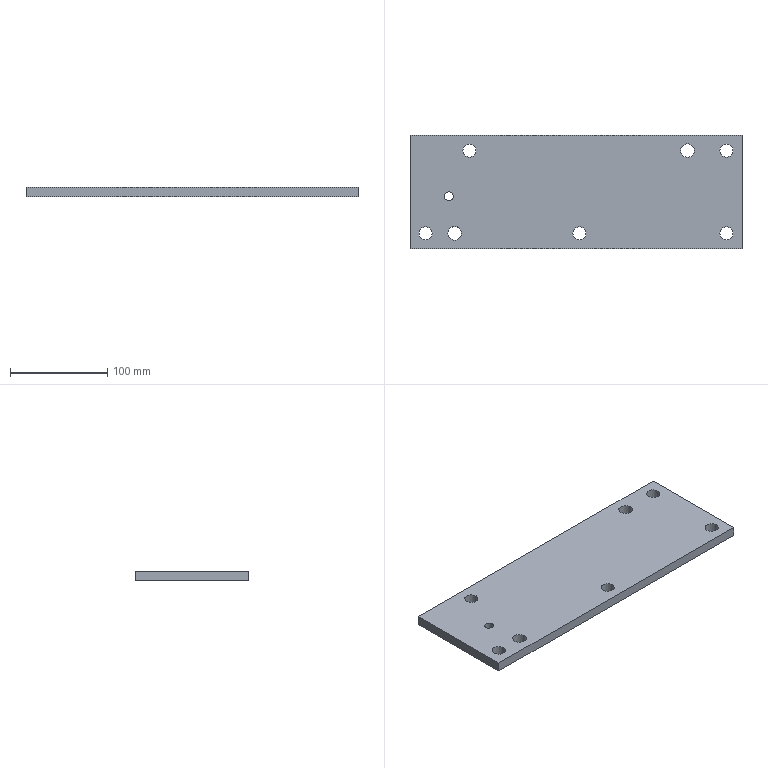Part | NX | features 6 2 | 1 solid | 14 faces | box 341 x 117 x 10 mm | volume 388098 mm3 | cylinder 8 | plane 6 | commonest cylinder face diameters 13.5 x5 14.001 x2 9 x1
STEP:
#1=CARTESIAN_POINT('',(339.11,437.223,91.));
#2=VERTEX_POINT('',#1);
#3=CARTESIAN_POINT('',(332.109,437.223,91.));
#4=DIRECTION('',(0.,0.,1.));
#5=DIRECTION('',(1.,0.,0.));
#6=AXIS2_PLACEMENT_3D('',#3,#4,#5);
#7=CIRCLE('',#6,7.);
#8=EDGE_CURVE('',#2,#2,#7,.T.);
#9=ORIENTED_EDGE('',*,*,#8,.T.);
#10=EDGE_LOOP('',(#9));
#11=FACE_BOUND('',#10,.T.);
#12=CARTESIAN_POINT('',(114.859,437.223,91.));
#13=VERTEX_POINT('',#12);
#14=CARTESIAN_POINT('',(108.109,437.223,91.));
#15=DIRECTION('',(0.,0.,1.));
#16=DIRECTION('',(1.,0.,0.));
#17=AXIS2_PLACEMENT_3D('',#14,#15,#16);
#18=CIRCLE('',#17,6.75);
#19=EDGE_CURVE('',#13,#13,#18,.T.);
#20=ORIENTED_EDGE('',*,*,#19,.T.);
#21=EDGE_LOOP('',(#20));
#22=FACE_BOUND('',#21,.T.);
#23=CARTESIAN_POINT('',(378.859,437.223,91.));
#24=VERTEX_POINT('',#23);
#25=CARTESIAN_POINT('',(372.109,437.223,91.));
#26=DIRECTION('',(0.,0.,1.));
#27=DIRECTION('',(1.,0.,0.));
#28=AXIS2_PLACEMENT_3D('',#25,#26,#27);
#29=CIRCLE('',#28,6.75);
#30=EDGE_CURVE('',#24,#24,#29,.T.);
#31=ORIENTED_EDGE('',*,*,#30,.T.);
#32=EDGE_LOOP('',(#31));
#33=FACE_BOUND('',#32,.T.);
#34=CARTESIAN_POINT('',(388.109,336.223,91.));
#35=VERTEX_POINT('',#34);
#36=CARTESIAN_POINT('',(388.109,453.223,91.));
#37=VERTEX_POINT('',#36);
#38=CARTESIAN_POINT('',(388.109,392.723,91.));
#39=DIRECTION('',(0.,1.,0.));
#40=VECTOR('',#39,1000.);
#41=LINE('',#38,#40);
#42=EDGE_CURVE('',#35,#37,#41,.T.);
#43=ORIENTED_EDGE('',*,*,#42,.F.);
#44=CARTESIAN_POINT('',(47.109,336.223,91.));
#45=VERTEX_POINT('',#44);
#46=CARTESIAN_POINT('',(245.109,336.223,91.));
#47=DIRECTION('',(1.,0.,0.));
#48=VECTOR('',#47,1000.);
#49=LINE('',#46,#48);
#50=EDGE_CURVE('',#45,#35,#49,.T.);
#51=ORIENTED_EDGE('',*,*,#50,.F.);
#52=CARTESIAN_POINT('',(47.109,453.223,91.));
#53=VERTEX_POINT('',#52);
#54=CARTESIAN_POINT('',(47.109,392.723,91.));
#55=DIRECTION('',(0.,-1.,0.));
#56=VECTOR('',#55,1000.);
#57=LINE('',#54,#56);
#58=EDGE_CURVE('',#53,#45,#57,.T.);
#59=ORIENTED_EDGE('',*,*,#58,.F.);
#60=CARTESIAN_POINT('',(245.109,453.223,91.));
#61=DIRECTION('',(-1.,0.,0.));
#62=VECTOR('',#61,1000.);
#63=LINE('',#60,#62);
#64=EDGE_CURVE('',#37,#53,#63,.T.);
#65=ORIENTED_EDGE('',*,*,#64,.F.);
#66=EDGE_LOOP('',(#43,#51,#59,#65));
#67=FACE_BOUND('',#66,.T.);
#68=CARTESIAN_POINT('',(69.859,352.223,91.));
#69=VERTEX_POINT('',#68);
#70=CARTESIAN_POINT('',(63.109,352.223,91.));
#71=DIRECTION('',(0.,0.,1.));
#72=DIRECTION('',(1.,0.,0.));
#73=AXIS2_PLACEMENT_3D('',#70,#71,#72);
#74=CIRCLE('',#73,6.75);
#75=EDGE_CURVE('',#69,#69,#74,.T.);
#76=ORIENTED_EDGE('',*,*,#75,.T.);
#77=EDGE_LOOP('',(#76));
#78=FACE_BOUND('',#77,.T.);
#79=CARTESIAN_POINT('',(378.859,352.223,91.));
#80=VERTEX_POINT('',#79);
#81=CARTESIAN_POINT('',(372.109,352.223,91.));
#82=DIRECTION('',(0.,0.,1.));
#83=DIRECTION('',(1.,0.,0.));
#84=AXIS2_PLACEMENT_3D('',#81,#82,#83);
#85=CIRCLE('',#84,6.75);
#86=EDGE_CURVE('',#80,#80,#85,.T.);
#87=ORIENTED_EDGE('',*,*,#86,.T.);
#88=EDGE_LOOP('',(#87));
#89=FACE_BOUND('',#88,.T.);
#90=CARTESIAN_POINT('',(100.11,352.223,91.));
#91=VERTEX_POINT('',#90);
#92=CARTESIAN_POINT('',(93.109,352.223,91.));
#93=DIRECTION('',(0.,0.,1.));
#94=DIRECTION('',(1.,0.,0.));
#95=AXIS2_PLACEMENT_3D('',#92,#93,#94);
#96=CIRCLE('',#95,7.);
#97=EDGE_CURVE('',#91,#91,#96,.T.);
#98=ORIENTED_EDGE('',*,*,#97,.T.);
#99=EDGE_LOOP('',(#98));
#100=FACE_BOUND('',#99,.T.);
#101=CARTESIAN_POINT('',(82.529,390.45,91.));
#102=VERTEX_POINT('',#101);
#103=CARTESIAN_POINT('',(87.029,390.45,91.));
#104=DIRECTION('',(0.,0.,-1.));
#105=DIRECTION('',(-1.,0.,0.));
#106=AXIS2_PLACEMENT_3D('',#103,#104,#105);
#107=CIRCLE('',#106,4.5);
#108=EDGE_CURVE('',#102,#102,#107,.T.);
#109=ORIENTED_EDGE('',*,*,#108,.F.);
#110=EDGE_LOOP('',(#109));
#111=FACE_BOUND('',#110,.T.);
#112=CARTESIAN_POINT('',(214.359,352.223,91.));
#113=VERTEX_POINT('',#112);
#114=CARTESIAN_POINT('',(221.109,352.223,91.));
#115=DIRECTION('',(0.,0.,-1.));
#116=DIRECTION('',(-1.,0.,0.));
#117=AXIS2_PLACEMENT_3D('',#114,#115,#116);
#118=CIRCLE('',#117,6.75);
#119=EDGE_CURVE('',#113,#113,#118,.T.);
#120=ORIENTED_EDGE('',*,*,#119,.F.);
#121=EDGE_LOOP('',(#120));
#122=FACE_BOUND('',#121,.T.);
#123=CARTESIAN_POINT('',(245.109,392.723,91.));
#124=DIRECTION('',(0.,0.,-1.));
#125=DIRECTION('',(1.,0.,0.));
#126=AXIS2_PLACEMENT_3D('',#123,#124,#125);
#127=PLANE('',#126);
#128=ADVANCED_FACE('',(#11,#22,#33,#67,#78,#89,#100,#111,#122),#127,.T.);
#129=CARTESIAN_POINT('',(339.11,437.223,101.));
#130=VERTEX_POINT('',#129);
#131=CARTESIAN_POINT('',(332.109,437.223,101.));
#132=DIRECTION('',(0.,0.,-1.));
#133=DIRECTION('',(1.,0.,0.));
#134=AXIS2_PLACEMENT_3D('',#131,#132,#133);
#135=CIRCLE('',#134,7.);
#136=EDGE_CURVE('',#130,#130,#135,.T.);
#137=ORIENTED_EDGE('',*,*,#136,.T.);
#138=EDGE_LOOP('',(#137));
#139=FACE_BOUND('',#138,.T.);
#140=CARTESIAN_POINT('',(114.859,437.223,101.));
#141=VERTEX_POINT('',#140);
#142=CARTESIAN_POINT('',(108.109,437.223,101.));
#143=DIRECTION('',(0.,0.,-1.));
#144=DIRECTION('',(1.,0.,0.));
#145=AXIS2_PLACEMENT_3D('',#142,#143,#144);
#146=CIRCLE('',#145,6.75);
#147=EDGE_CURVE('',#141,#141,#146,.T.);
#148=ORIENTED_EDGE('',*,*,#147,.T.);
#149=EDGE_LOOP('',(#148));
#150=FACE_BOUND('',#149,.T.);
#151=CARTESIAN_POINT('',(378.859,437.223,101.));
#152=VERTEX_POINT('',#151);
#153=CARTESIAN_POINT('',(372.109,437.223,101.));
#154=DIRECTION('',(0.,0.,-1.));
#155=DIRECTION('',(1.,0.,0.));
#156=AXIS2_PLACEMENT_3D('',#153,#154,#155);
#157=CIRCLE('',#156,6.75);
#158=EDGE_CURVE('',#152,#152,#157,.T.);
#159=ORIENTED_EDGE('',*,*,#158,.T.);
#160=EDGE_LOOP('',(#159));
#161=FACE_BOUND('',#160,.T.);
#162=CARTESIAN_POINT('',(388.109,336.223,101.));
#163=VERTEX_POINT('',#162);
#164=CARTESIAN_POINT('',(47.109,336.223,101.));
#165=VERTEX_POINT('',#164);
#166=CARTESIAN_POINT('',(245.109,336.223,101.));
#167=DIRECTION('',(-1.,0.,0.));
#168=VECTOR('',#167,1000.);
#169=LINE('',#166,#168);
#170=EDGE_CURVE('',#163,#165,#169,.T.);
#171=ORIENTED_EDGE('',*,*,#170,.F.);
#172=CARTESIAN_POINT('',(388.109,453.223,101.));
#173=VERTEX_POINT('',#172);
#174=CARTESIAN_POINT('',(388.109,392.723,101.));
#175=DIRECTION('',(0.,-1.,0.));
#176=VECTOR('',#175,1000.);
#177=LINE('',#174,#176);
#178=EDGE_CURVE('',#173,#163,#177,.T.);
#179=ORIENTED_EDGE('',*,*,#178,.F.);
#180=CARTESIAN_POINT('',(47.109,453.223,101.));
#181=VERTEX_POINT('',#180);
#182=CARTESIAN_POINT('',(245.109,453.223,101.));
#183=DIRECTION('',(1.,0.,0.));
#184=VECTOR('',#183,1000.);
#185=LINE('',#182,#184);
#186=EDGE_CURVE('',#181,#173,#185,.T.);
#187=ORIENTED_EDGE('',*,*,#186,.F.);
#188=CARTESIAN_POINT('',(47.109,392.723,101.));
#189=DIRECTION('',(0.,1.,0.));
#190=VECTOR('',#189,1000.);
#191=LINE('',#188,#190);
#192=EDGE_CURVE('',#165,#181,#191,.T.);
#193=ORIENTED_EDGE('',*,*,#192,.F.);
#194=EDGE_LOOP('',(#171,#179,#187,#193));
#195=FACE_BOUND('',#194,.T.);
#196=CARTESIAN_POINT('',(69.859,352.223,101.));
#197=VERTEX_POINT('',#196);
#198=CARTESIAN_POINT('',(63.109,352.223,101.));
#199=DIRECTION('',(0.,0.,-1.));
#200=DIRECTION('',(1.,0.,0.));
#201=AXIS2_PLACEMENT_3D('',#198,#199,#200);
#202=CIRCLE('',#201,6.75);
#203=EDGE_CURVE('',#197,#197,#202,.T.);
#204=ORIENTED_EDGE('',*,*,#203,.T.);
#205=EDGE_LOOP('',(#204));
#206=FACE_BOUND('',#205,.T.);
#207=CARTESIAN_POINT('',(378.859,352.223,101.));
#208=VERTEX_POINT('',#207);
#209=CARTESIAN_POINT('',(372.109,352.223,101.));
#210=DIRECTION('',(0.,0.,-1.));
#211=DIRECTION('',(1.,0.,0.));
#212=AXIS2_PLACEMENT_3D('',#209,#210,#211);
#213=CIRCLE('',#212,6.75);
#214=EDGE_CURVE('',#208,#208,#213,.T.);
#215=ORIENTED_EDGE('',*,*,#214,.T.);
#216=EDGE_LOOP('',(#215));
#217=FACE_BOUND('',#216,.T.);
#218=CARTESIAN_POINT('',(100.11,352.223,101.));
#219=VERTEX_POINT('',#218);
#220=CARTESIAN_POINT('',(93.109,352.223,101.));
#221=DIRECTION('',(0.,0.,-1.));
#222=DIRECTION('',(1.,0.,0.));
#223=AXIS2_PLACEMENT_3D('',#220,#221,#222);
#224=CIRCLE('',#223,7.);
#225=EDGE_CURVE('',#219,#219,#224,.T.);
#226=ORIENTED_EDGE('',*,*,#225,.T.);
#227=EDGE_LOOP('',(#226));
#228=FACE_BOUND('',#227,.T.);
#229=CARTESIAN_POINT('',(91.529,390.45,101.));
#230=VERTEX_POINT('',#229);
#231=CARTESIAN_POINT('',(87.029,390.45,101.));
#232=DIRECTION('',(0.,0.,-1.));
#233=DIRECTION('',(1.,0.,0.));
#234=AXIS2_PLACEMENT_3D('',#231,#232,#233);
#235=CIRCLE('',#234,4.5);
#236=EDGE_CURVE('',#230,#230,#235,.T.);
#237=ORIENTED_EDGE('',*,*,#236,.T.);
#238=EDGE_LOOP('',(#237));
#239=FACE_BOUND('',#238,.T.);
#240=CARTESIAN_POINT('',(227.859,352.223,101.));
#241=VERTEX_POINT('',#240);
#242=CARTESIAN_POINT('',(221.109,352.223,101.));
#243=DIRECTION('',(0.,0.,1.));
#244=DIRECTION('',(1.,0.,0.));
#245=AXIS2_PLACEMENT_3D('',#242,#243,#244);
#246=CIRCLE('',#245,6.75);
#247=EDGE_CURVE('',#241,#241,#246,.T.);
#248=ORIENTED_EDGE('',*,*,#247,.F.);
#249=EDGE_LOOP('',(#248));
#250=FACE_BOUND('',#249,.T.);
#251=CARTESIAN_POINT('',(-461.37,123.939,101.));
#252=DIRECTION('',(0.,0.,1.));
#253=DIRECTION('',(-1.,0.,0.));
#254=AXIS2_PLACEMENT_3D('',#251,#252,#253);
#255=PLANE('',#254);
#256=ADVANCED_FACE('',(#139,#150,#161,#195,#206,#217,#228,#239,#250),#255,.T.);
#257=ORIENTED_EDGE('',*,*,#136,.F.);
#258=EDGE_LOOP('',(#257));
#259=FACE_BOUND('',#258,.T.);
#260=ORIENTED_EDGE('',*,*,#8,.F.);
#261=EDGE_LOOP('',(#260));
#262=FACE_BOUND('',#261,.T.);
#263=CARTESIAN_POINT('',(332.109,437.223,91.));
#264=DIRECTION('',(0.,0.,1.));
#265=DIRECTION('',(-1.,0.,0.));
#266=AXIS2_PLACEMENT_3D('',#263,#264,#265);
#267=CYLINDRICAL_SURFACE('',#266,7.);
#268=ADVANCED_FACE('',(#259,#262),#267,.F.);
#269=ORIENTED_EDGE('',*,*,#147,.F.);
#270=EDGE_LOOP('',(#269));
#271=FACE_BOUND('',#270,.T.);
#272=ORIENTED_EDGE('',*,*,#19,.F.);
#273=EDGE_LOOP('',(#272));
#274=FACE_BOUND('',#273,.T.);
#275=CARTESIAN_POINT('',(108.109,437.223,91.));
#276=DIRECTION('',(0.,0.,1.));
#277=DIRECTION('',(-1.,0.,0.));
#278=AXIS2_PLACEMENT_3D('',#275,#276,#277);
#279=CYLINDRICAL_SURFACE('',#278,6.75);
#280=ADVANCED_FACE('',(#271,#274),#279,.F.);
#281=ORIENTED_EDGE('',*,*,#158,.F.);
#282=EDGE_LOOP('',(#281));
#283=FACE_BOUND('',#282,.T.);
#284=ORIENTED_EDGE('',*,*,#30,.F.);
#285=EDGE_LOOP('',(#284));
#286=FACE_BOUND('',#285,.T.);
#287=CARTESIAN_POINT('',(372.109,437.223,91.));
#288=DIRECTION('',(0.,0.,1.));
#289=DIRECTION('',(-1.,0.,0.));
#290=AXIS2_PLACEMENT_3D('',#287,#288,#289);
#291=CYLINDRICAL_SURFACE('',#290,6.75);
#292=ADVANCED_FACE('',(#283,#286),#291,.F.);
#293=CARTESIAN_POINT('',(47.109,453.223,91.));
#294=DIRECTION('',(0.,0.,1.));
#295=VECTOR('',#294,1000.);
#296=LINE('',#293,#295);
#297=EDGE_CURVE('',#53,#181,#296,.T.);
#298=ORIENTED_EDGE('',*,*,#297,.T.);
#299=ORIENTED_EDGE('',*,*,#186,.T.);
#300=CARTESIAN_POINT('',(388.109,453.223,91.));
#301=DIRECTION('',(0.,0.,1.));
#302=VECTOR('',#301,1000.);
#303=LINE('',#300,#302);
#304=EDGE_CURVE('',#37,#173,#303,.T.);
#305=ORIENTED_EDGE('',*,*,#304,.F.);
#306=ORIENTED_EDGE('',*,*,#64,.T.);
#307=EDGE_LOOP('',(#298,#299,#305,#306));
#308=FACE_BOUND('',#307,.T.);
#309=CARTESIAN_POINT('',(245.109,453.223,91.));
#310=DIRECTION('',(0.,1.,0.));
#311=DIRECTION('',(0.,0.,-1.));
#312=AXIS2_PLACEMENT_3D('',#309,#310,#311);
#313=PLANE('',#312);
#314=ADVANCED_FACE('',(#308),#313,.T.);
#315=CARTESIAN_POINT('',(47.109,336.223,91.));
#316=DIRECTION('',(0.,0.,1.));
#317=VECTOR('',#316,1000.);
#318=LINE('',#315,#317);
#319=EDGE_CURVE('',#45,#165,#318,.T.);
#320=ORIENTED_EDGE('',*,*,#319,.T.);
#321=ORIENTED_EDGE('',*,*,#192,.T.);
#322=ORIENTED_EDGE('',*,*,#297,.F.);
#323=ORIENTED_EDGE('',*,*,#58,.T.);
#324=EDGE_LOOP('',(#320,#321,#322,#323));
#325=FACE_BOUND('',#324,.T.);
#326=CARTESIAN_POINT('',(47.109,392.723,91.));
#327=DIRECTION('',(-1.,0.,0.));
#328=DIRECTION('',(0.,0.,-1.));
#329=AXIS2_PLACEMENT_3D('',#326,#327,#328);
#330=PLANE('',#329);
#331=ADVANCED_FACE('',(#325),#330,.T.);
#332=CARTESIAN_POINT('',(388.109,336.223,91.));
#333=DIRECTION('',(0.,0.,1.));
#334=VECTOR('',#333,1000.);
#335=LINE('',#332,#334);
#336=EDGE_CURVE('',#35,#163,#335,.T.);
#337=ORIENTED_EDGE('',*,*,#336,.T.);
#338=ORIENTED_EDGE('',*,*,#170,.T.);
#339=ORIENTED_EDGE('',*,*,#319,.F.);
#340=ORIENTED_EDGE('',*,*,#50,.T.);
#341=EDGE_LOOP('',(#337,#338,#339,#340));
#342=FACE_BOUND('',#341,.T.);
#343=CARTESIAN_POINT('',(245.109,336.223,91.));
#344=DIRECTION('',(0.,-1.,0.));
#345=DIRECTION('',(0.,0.,1.));
#346=AXIS2_PLACEMENT_3D('',#343,#344,#345);
#347=PLANE('',#346);
#348=ADVANCED_FACE('',(#342),#347,.T.);
#349=ORIENTED_EDGE('',*,*,#42,.T.);
#350=ORIENTED_EDGE('',*,*,#304,.T.);
#351=ORIENTED_EDGE('',*,*,#178,.T.);
#352=ORIENTED_EDGE('',*,*,#336,.F.);
#353=EDGE_LOOP('',(#349,#350,#351,#352));
#354=FACE_BOUND('',#353,.T.);
#355=CARTESIAN_POINT('',(388.109,392.723,91.));
#356=DIRECTION('',(1.,0.,0.));
#357=DIRECTION('',(0.,0.,1.));
#358=AXIS2_PLACEMENT_3D('',#355,#356,#357);
#359=PLANE('',#358);
#360=ADVANCED_FACE('',(#354),#359,.T.);
#361=ORIENTED_EDGE('',*,*,#203,.F.);
#362=EDGE_LOOP('',(#361));
#363=FACE_BOUND('',#362,.T.);
#364=ORIENTED_EDGE('',*,*,#75,.F.);
#365=EDGE_LOOP('',(#364));
#366=FACE_BOUND('',#365,.T.);
#367=CARTESIAN_POINT('',(63.109,352.223,91.));
#368=DIRECTION('',(0.,0.,1.));
#369=DIRECTION('',(-1.,0.,0.));
#370=AXIS2_PLACEMENT_3D('',#367,#368,#369);
#371=CYLINDRICAL_SURFACE('',#370,6.75);
#372=ADVANCED_FACE('',(#363,#366),#371,.F.);
#373=ORIENTED_EDGE('',*,*,#214,.F.);
#374=EDGE_LOOP('',(#373));
#375=FACE_BOUND('',#374,.T.);
#376=ORIENTED_EDGE('',*,*,#86,.F.);
#377=EDGE_LOOP('',(#376));
#378=FACE_BOUND('',#377,.T.);
#379=CARTESIAN_POINT('',(372.109,352.223,91.));
#380=DIRECTION('',(0.,0.,1.));
#381=DIRECTION('',(-1.,0.,0.));
#382=AXIS2_PLACEMENT_3D('',#379,#380,#381);
#383=CYLINDRICAL_SURFACE('',#382,6.75);
#384=ADVANCED_FACE('',(#375,#378),#383,.F.);
#385=ORIENTED_EDGE('',*,*,#225,.F.);
#386=EDGE_LOOP('',(#385));
#387=FACE_BOUND('',#386,.T.);
#388=ORIENTED_EDGE('',*,*,#97,.F.);
#389=EDGE_LOOP('',(#388));
#390=FACE_BOUND('',#389,.T.);
#391=CARTESIAN_POINT('',(93.109,352.223,91.));
#392=DIRECTION('',(0.,0.,1.));
#393=DIRECTION('',(-1.,0.,0.));
#394=AXIS2_PLACEMENT_3D('',#391,#392,#393);
#395=CYLINDRICAL_SURFACE('',#394,7.);
#396=ADVANCED_FACE('',(#387,#390),#395,.F.);
#397=ORIENTED_EDGE('',*,*,#236,.F.);
#398=EDGE_LOOP('',(#397));
#399=FACE_BOUND('',#398,.T.);
#400=ORIENTED_EDGE('',*,*,#108,.T.);
#401=EDGE_LOOP('',(#400));
#402=FACE_BOUND('',#401,.T.);
#403=CARTESIAN_POINT('',(87.029,390.45,-71.));
#404=DIRECTION('',(0.,0.,1.));
#405=DIRECTION('',(-1.,0.,0.));
#406=AXIS2_PLACEMENT_3D('',#403,#404,#405);
#407=CYLINDRICAL_SURFACE('',#406,4.5);
#408=ADVANCED_FACE('',(#399,#402),#407,.F.);
#409=ORIENTED_EDGE('',*,*,#247,.T.);
#410=EDGE_LOOP('',(#409));
#411=FACE_BOUND('',#410,.T.);
#412=ORIENTED_EDGE('',*,*,#119,.T.);
#413=EDGE_LOOP('',(#412));
#414=FACE_BOUND('',#413,.T.);
#415=CARTESIAN_POINT('',(221.109,352.223,91.));
#416=DIRECTION('',(0.,0.,1.));
#417=DIRECTION('',(-1.,0.,0.));
#418=AXIS2_PLACEMENT_3D('',#415,#416,#417);
#419=CYLINDRICAL_SURFACE('',#418,6.75);
#420=ADVANCED_FACE('',(#411,#414),#419,.F.);
#421=CLOSED_SHELL('',(#128,#256,#268,#280,#292,#314,#331,#348,#360,#372,#384,#396,#408,#420));
#422=MANIFOLD_SOLID_BREP('',#421);
#423=(LENGTH_UNIT()NAMED_UNIT(*)SI_UNIT(.MILLI.,.METRE.));
#424=UNCERTAINTY_MEASURE_WITH_UNIT(LENGTH_MEASURE(0.00001),#423,'','');
#425=(NAMED_UNIT(*)PLANE_ANGLE_UNIT()SI_UNIT($,.RADIAN.));
#426=(NAMED_UNIT(*)SI_UNIT($,.STERADIAN.)SOLID_ANGLE_UNIT());
#427=(GEOMETRIC_REPRESENTATION_CONTEXT(3)GLOBAL_UNCERTAINTY_ASSIGNED_CONTEXT((#424))GLOBAL_UNIT_ASSIGNED_CONTEXT((#423,#425,#426))REPRESENTATION_CONTEXT('',''));
#428=ADVANCED_BREP_SHAPE_REPRESENTATION('',(#422),#427);